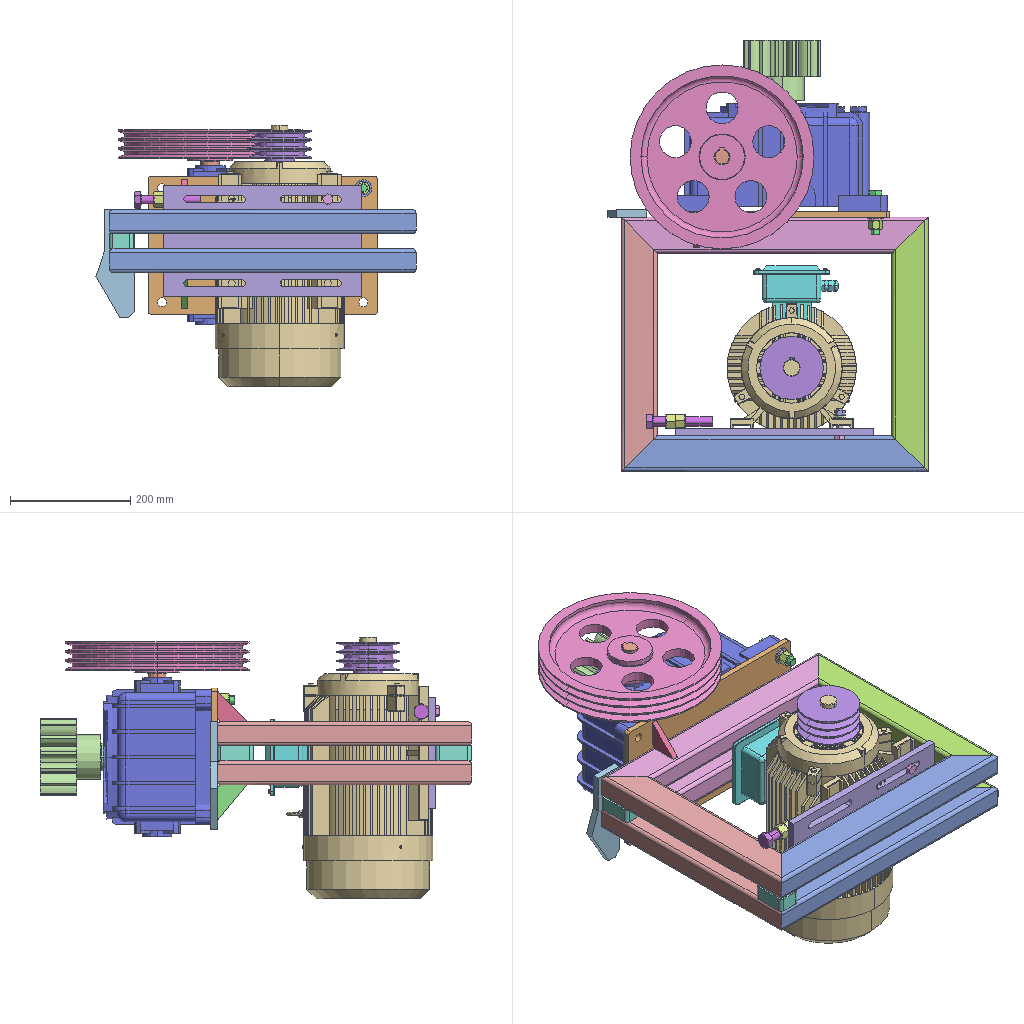Assembly | SolidWorks | 25 different items | 28 placed | box 532 x 717 x 435 mm
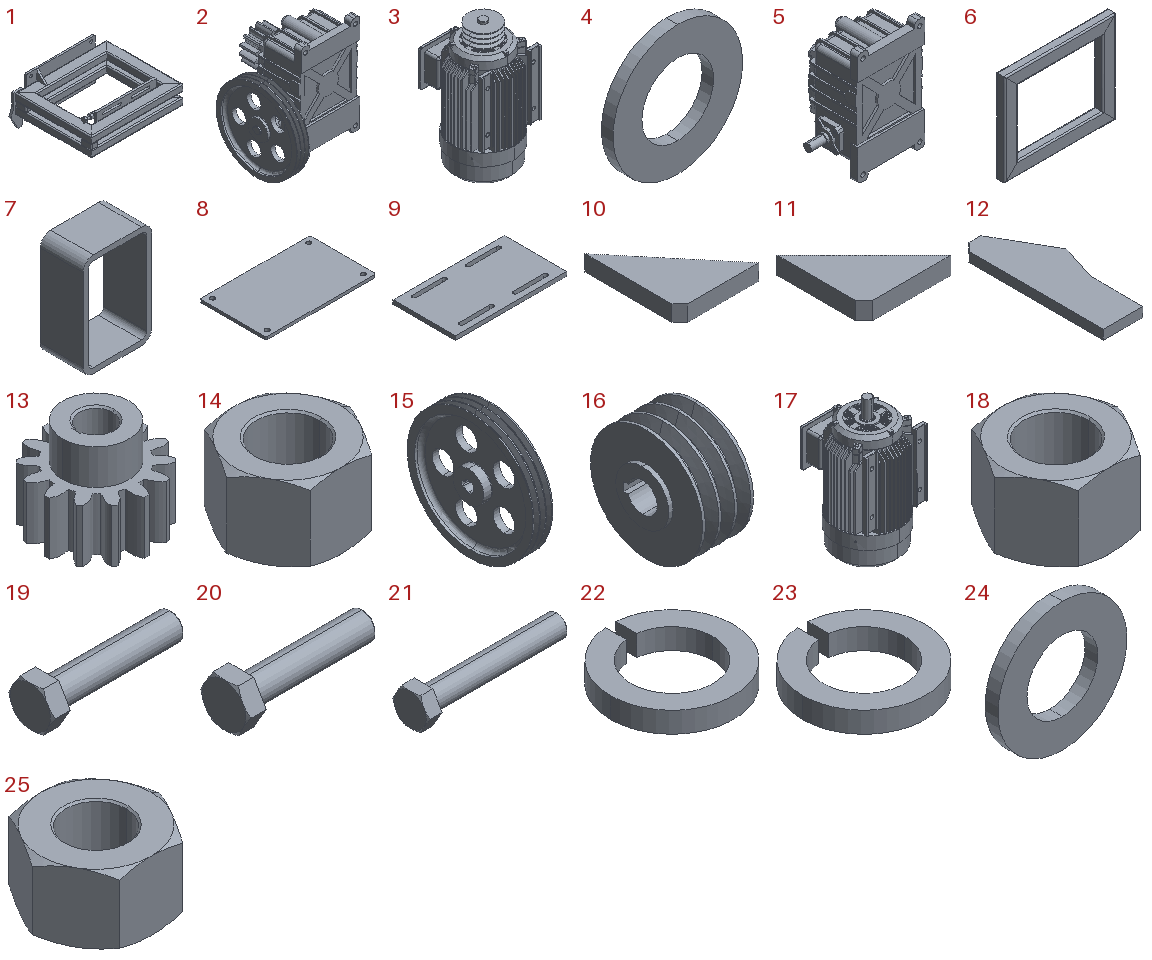Parts list (item | name | quantity | parent item | size | volume | features):
1 | (subassembly) | x1 | - | 532.27 x 435 x 236 mm | 3498910 mm3 | -
2 | (subassembly) | x1 | - | 324 x 347 x 428.15 mm | 12606239 mm3 | features CompositeCurve 1
3 | (subassembly) | x1 | - | 215 x 277.5 x 435 mm | 11973483 mm3 | -
4 | - | x1 | - | 28 x 2.5 x 28 mm | 1068 mm3 | features Revolution 1
5 | - | x1 | in 2 | 322 x 259 x 375 mm | 10630129 mm3 | features ICE 22, DeleteBody 4, Fillet 4, LPattern 3, MirrorSolid 3, Chamfer 2, CirPattern 2, Revolution 2, CombineBodies 1, Extrusion 1, MirrorPattern 1, RevCut 1
6 | - | x2 | in 1 | 510 x 40 x 423 mm | 879378 mm3 | features WeldMemberFeat 1, WeldmentFeature 1
7 | - | x2 | in 1 | 40 x 25 x 60 mm | 13521 mm3 | features WeldMemberFeat 1, WeldmentFeature 1
8 | - | x1 | in 1 | 381 x 230 x 10 mm | 869017 mm3 | features Chamfer 1, Extrusion 1, Fillet 1, HoleWzd 1
9 | - | x1 | in 1 | 330 x 185 x 12 mm | 675331 mm3 | features Chamfer 1, Extrusion 1, HoleWzd 1
10 | - | x1 | in 1 | 50 x 60 x 10 mm | 14875 mm3 | features Chamfer 1, Extrusion 1
11 | - | x1 | in 1 | 50 x 50 x 10 mm | 12375 mm3 | features Chamfer 1, Extrusion 1
12 | - | x1 | in 1 | 64.77 x 180 x 12 mm | 107100 mm3 | features Chamfer 1, Extrusion 1
13 | - | x1 | in 2 | 127.519 x 127.793 x 100 mm | 607149 mm3 | features ICE 4, Chamfer 1, CirPattern 1, Extrusion 1
14 | - | x1 | - | 22.8 x 19.745 x 13.9 mm | 3143 mm3 | features Cut 2, Chamfer 1, Extrusion 1
15 | - | x1 | in 2 | 52 x 306 x 306 mm | 1368961 mm3 | features ICE 6, Chamfer 2, CirPattern 1, Fillet 1, Revolution 1
16 | - | x1 | in 3 | 52 x 105.5 x 105.5 mm | 299364 mm3 | features ICE 2, Revolution 1
17 | - | x1 | in 3 | 215 x 277.5 x 435 mm | 11674119 mm3 | features ICE 34, Fillet 14, CirPattern 7, Revolution 6, Chamfer 4, Extrusion 4, Dome 3, DeleteBody 2, RefAxis 2, MirrorPattern 1, MirrorSolid 1, MoveCopyBody 1, RevCut 1
18 | - | x2 | in 1 | 26.2 x 22.69 x 15.9 mm | 4666 mm3 | features Cut 2, Chamfer 1, Extrusion 1
19 | - | x1 | - | 73.8 x 24.249 x 21 mm | 13362 mm3 | features Chamfer 2, RevCut 2, Revolution 2, Extrusion 1, ICE 1
20 | - | x1 | - | 51.4 x 18.475 x 16 mm | 4953 mm3 | features Chamfer 2, RevCut 2, Revolution 2, Extrusion 1, ICE 1
21 | - | x1 | in 1 | 110 x 27.713 x 24 mm | 25081 mm3 | features Chamfer 2, RevCut 2, Revolution 2, Extrusion 1, ICE 1
22 | - | x1 | - | 21.361 x 21.323 x 3.6 mm | 696.819 mm3 | features Extrusion 1
23 | - | x1 | - | 15.372 x 15.344 x 2.6 mm | 261.313 mm3 | features Extrusion 1
24 | - | x1 | - | 20 x 2 x 20 mm | 438.252 mm3 | features Revolution 1
25 | - | x1 | - | 17.6 x 15.242 x 9.5 mm | 1379 mm3 | features Cut 2, Chamfer 1, Extrusion 1
Mates (type | each side: item.copy, entity, surface, feature):
In the top assembly
Coincident | 9.1 face plane Boss-Extrude1 | 17.1 face plane Boss-Extrude19
Slot | 17.1 face cylinder Cut-Extrude15 | 9.1 face plane Ø22 Hole1
Parallel | 9.1 face plane Boss-Extrude1 | 17.1 face plane Boss-Extrude19
Coincident | 8.1 face plane Boss-Extrude1 | 5.1 face plane Boss-Extrude2
Concentric | 8.1 face cylinder Ø15 Hole1 | 5.1 face cylinder Boss-Extrude2 | 2 times
Concentric | 19.1 face cylinder Revolve1 | 22.1 face cylinder Extrude1
Concentric | 22.1 face cylinder Extrude1 | 4.1 face cylinder Revolve
Concentric | 22.1 face cylinder Extrude1 | 14.1 face cylinder Boss-Extrude
Coincident | 22.1 face plane Extrude1 | 4.1 face plane Revolve
Coincident | 22.1 face plane Extrude1 | 14.1 face plane Boss-Extrude
Concentric | 5.1 face cylinder Boss-Extrude2 | 19.1 face cylinder Revolve1
Coincident | 5.1 face plane Boss-Extrude2 | 19.1 face plane Boss-Extrude1
Coincident | 8.1 face plane Boss-Extrude1 | 4.1 face plane Revolve
Concentric | 20.1 face cylinder Revolve1 | 23.1 face cylinder Extrude1
Concentric | 24.1 face cylinder Revolve | 25.1 face cylinder Boss-Extrude
Concentric | 20.1 face cylinder Revolve1 | 25.1 face cylinder Boss-Extrude
Coincident | 23.1 face plane Extrude1 | 25.1 face plane Boss-Extrude
Coincident | 23.1 face plane Extrude1 | 24.1 face plane Revolve
Concentric | 17.1 face cylinder Cut-Extrude15 | 20.1 face cylinder Revolve1
Coincident | 17.1 face plane Boss-Extrude19 | 24.1 face plane Revolve
Coincident | 9.1 face plane Boss-Extrude1 | 20.1 face plane Boss-Extrude1
In subassembly 2
Concentric | 5.2 face cylinder Revolve1 | 13.1 edge
Coincident | 5.2 face plane Boss-Extrude19 | 13.1 face plane Cut-Extrude2
DistanceDim | 13.1 face plane Boss-Extrude1 | 5.2 face plane Boss-Extrude2
Concentric | 5.2 face cylinder Mirror4 | 15.1 face cylinder Revolve1
Coincident | 5.2 face plane Mirror4 | 15.1 face plane Boss-Extrude2
In subassembly 3
Concentric | 17.2 face cylinder Revolve1 | 16.1 face cylinder Revolve1
Parallel | 17.2 face plane Cut-Extrude12 | 16.1 face plane Cut-Extrude5
Coincident | 17.2 face plane Revolve1 | 16.1 face plane Boss-Extrude2
In subassembly 1
Coincident | 6.1 plane | 1.1 plane
Coincident | 6.1 face plane GB/T 6728-2002 Rectangular Hollow Section 60X40X3(1) | 1.1 plane
Coincident | 6.1 face plane GB/T 6728-2002 Rectangular Hollow Section 60X40X3(1) | 8.2 face plane Boss-Extrude1
Coincident | 8.2 plane | 1.1 plane
Coincident | 8.2 face plane Boss-Extrude1 | 10.1 face plane Boss-Extrude1
Coincident | 6.1 face plane GB/T 6728-2002 Rectangular Hollow Section 60X40X3(1) | 10.1 face plane Boss-Extrude1
Coincident | 6.1 face plane GB/T 6728-2002 Rectangular Hollow Section 60X40X3(1) | 12.1 face plane Boss-Extrude1
DistanceDim | 8.2 face plane Boss-Extrude1 | 12.1 face plane Boss-Extrude1
Coincident | 6.1 face plane GB/T 6728-2002 Rectangular Hollow Section 60X40X3(1) | 9.2 face plane Boss-Extrude1
Width | 9.2 face plane Boss-Extrude1 | 9.2 face plane Boss-Extrude1 | 8.2 face plane Boss-Extrude1 | 8.2 face plane Boss-Extrude1
DistanceDim | 6.1 face plane GB/T 6728-2002 Rectangular Hollow Section 60X40X3(1) | 10.1 face plane Boss-Extrude1
Coincident | 10.1 face plane Boss-Extrude1 | 11.1 face plane Boss-Extrude1
Coincident | 8.2 face plane Boss-Extrude1 | 11.1 face plane Boss-Extrude1
Symmetric | 7.1 face plane GB/T 6728-2002 Rectangular Hollow Section 60X40X3(1) | 7.1 face plane GB/T 6728-2002 Rectangular Hollow Section 60X40X3(1) | 1.1 plane
Coincident | 6.1 face plane GB/T 6728-2002 Rectangular Hollow Section 60X40X3(1) | 7.1 face plane GB/T 6728-2002 Rectangular Hollow Section 60X40X3(1) | 2 times
Coincident | 7.1 face plane GB/T 6728-2002 Rectangular Hollow Section 60X40X3(1) | 6.2 face plane GB/T 6728-2002 Rectangular Hollow Section 60X40X3(1) | 2 times
Coincident | 6.1 face plane GB/T 6728-2002 Rectangular Hollow Section 60X40X3(1) | 6.2 face plane GB/T 6728-2002 Rectangular Hollow Section 60X40X3(1) | 2 times
Coincident | 7.1 face plane GB/T 6728-2002 Rectangular Hollow Section 60X40X3(1) | 7.2 face plane GB/T 6728-2002 Rectangular Hollow Section 60X40X3(1)
Coincident | 7.1 face plane GB/T 6728-2002 Rectangular Hollow Section 60X40X3(1) | 7.2 edge
Coincident | 6.2 face plane GB/T 6728-2002 Rectangular Hollow Section 60X40X3(1) | 7.2 face plane GB/T 6728-2002 Rectangular Hollow Section 60X40X3(1)
Coincident | 12.1 face plane Boss-Extrude1 | 6.2 face plane GB/T 6728-2002 Rectangular Hollow Section 60X40X3(1)
DistanceDim | 8.2 face plane Boss-Extrude1 | 6.2 face plane GB/T 6728-2002 Rectangular Hollow Section 60X40X3(1)
Coincident | 11.1 face plane Boss-Extrude1 | 6.2 face plane GB/T 6728-2002 Rectangular Hollow Section 60X40X3(1)
Concentric | 18.1 face cylinder Boss-Extrude | 18.2 face cylinder Boss-Extrude
Coincident | 18.1 face plane Boss-Extrude | 18.2 face plane Boss-Extrude
Concentric | 18.1 face cylinder Boss-Extrude | 21.1 face cylinder Revolve1
Coincident | 9.2 face plane Boss-Extrude1 | 18.1 face plane Boss-Extrude
Coincident | 9.2 plane | 1.1 plane
Coincident | 9.2 face plane Boss-Extrude1 | 18.2 face plane Boss-Extrude
DistanceDim | 21.1 face plane Boss-Extrude1 | 6.2 face plane GB/T 6728-2002 Rectangular Hollow Section 60X40X3(1)
DistanceDim | 21.1 face cylinder Revolve1 | 6.2 face plane GB/T 6728-2002 Rectangular Hollow Section 60X40X3(1)
Parallel | 18.1 face plane Boss-Extrude | 21.1 face plane Boss-Extrude1